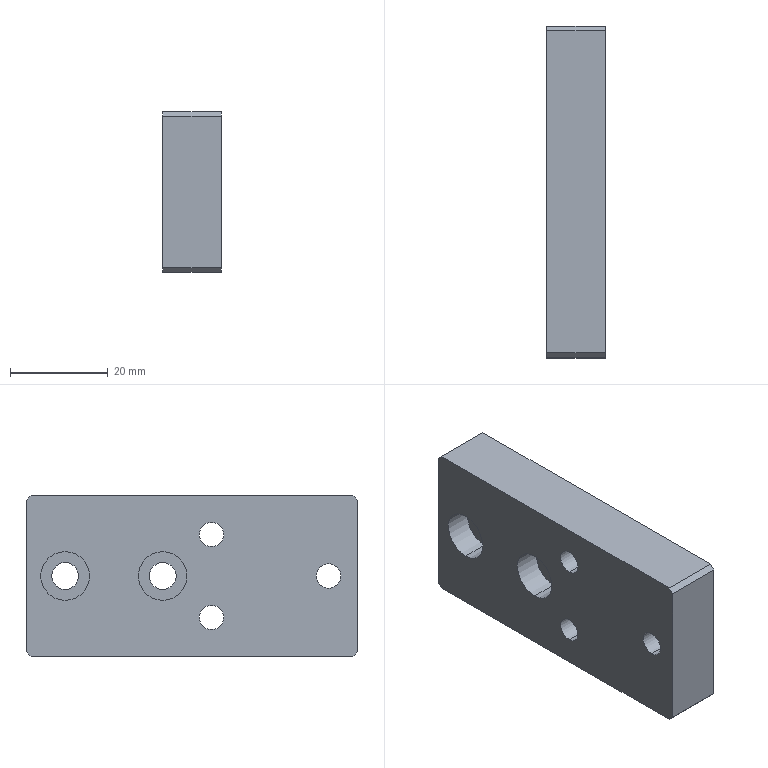Part | SolidWorks | features HoleWzd 3, Chamfer 1, Extrusion 1 | 1 solid | 34 faces | box 12 x 68 x 33 mm | volume 24708 mm3 | cylinder 18 | plane 12 | cone 4 | commonest cylinder face diameters 5 x6 4.2 x4 5.5 x4 10 x4
STEP:
#1=CARTESIAN_POINT('',(-70.982,-19.604,-21.5));
#2=VERTEX_POINT('',#1);
#3=CARTESIAN_POINT('',(-70.982,-19.604,-11.5));
#4=VERTEX_POINT('',#3);
#5=CARTESIAN_POINT('',(-70.982,-19.604,-16.5));
#6=DIRECTION('',(-1.,0.,0.));
#7=DIRECTION('',(0.,0.,1.));
#8=AXIS2_PLACEMENT_3D('',#5,#6,#7);
#9=CIRCLE('',#8,5.);
#10=EDGE_CURVE('',#2,#4,#9,.T.);
#11=ORIENTED_EDGE('',*,*,#10,.F.);
#12=CARTESIAN_POINT('',(-76.482,-19.604,-21.5));
#13=VERTEX_POINT('',#12);
#14=CARTESIAN_POINT('',(-76.482,-19.604,-21.5));
#15=DIRECTION('',(-1.,0.,0.));
#16=VECTOR('',#15,1000.);
#17=LINE('',#14,#16);
#18=EDGE_CURVE('',#2,#13,#17,.T.);
#19=ORIENTED_EDGE('',*,*,#18,.T.);
#20=CARTESIAN_POINT('',(-76.482,-19.604,-11.5));
#21=VERTEX_POINT('',#20);
#22=CARTESIAN_POINT('',(-76.482,-19.604,-16.5));
#23=DIRECTION('',(-1.,0.,0.));
#24=DIRECTION('',(0.,0.,1.));
#25=AXIS2_PLACEMENT_3D('',#22,#23,#24);
#26=CIRCLE('',#25,5.);
#27=EDGE_CURVE('',#13,#21,#26,.T.);
#28=ORIENTED_EDGE('',*,*,#27,.T.);
#29=CARTESIAN_POINT('',(-76.482,-19.604,-11.5));
#30=DIRECTION('',(-1.,0.,0.));
#31=VECTOR('',#30,1000.);
#32=LINE('',#29,#31);
#33=EDGE_CURVE('',#4,#21,#32,.T.);
#34=ORIENTED_EDGE('',*,*,#33,.F.);
#35=EDGE_LOOP('',(#11,#19,#28,#34));
#36=FACE_OUTER_BOUND('',#35,.T.);
#37=CARTESIAN_POINT('',(-76.482,-19.604,-16.5));
#38=DIRECTION('',(-1.,0.,0.));
#39=DIRECTION('',(0.,0.,1.));
#40=AXIS2_PLACEMENT_3D('',#37,#38,#39);
#41=CYLINDRICAL_SURFACE('',#40,5.);
#42=ADVANCED_FACE('',(#36),#41,.F.);
#43=CARTESIAN_POINT('',(-64.482,-19.604,-19.25));
#44=VERTEX_POINT('',#43);
#45=CARTESIAN_POINT('',(-64.482,-19.604,-13.75));
#46=VERTEX_POINT('',#45);
#47=CARTESIAN_POINT('',(-64.482,-19.604,-16.5));
#48=DIRECTION('',(-1.,0.,0.));
#49=DIRECTION('',(0.,0.,1.));
#50=AXIS2_PLACEMENT_3D('',#47,#48,#49);
#51=CIRCLE('',#50,2.75);
#52=EDGE_CURVE('',#44,#46,#51,.T.);
#53=ORIENTED_EDGE('',*,*,#52,.F.);
#54=CARTESIAN_POINT('',(-70.982,-19.604,-19.25));
#55=VERTEX_POINT('',#54);
#56=CARTESIAN_POINT('',(-76.482,-19.604,-19.25));
#57=DIRECTION('',(-1.,0.,0.));
#58=VECTOR('',#57,1000.);
#59=LINE('',#56,#58);
#60=EDGE_CURVE('',#44,#55,#59,.T.);
#61=ORIENTED_EDGE('',*,*,#60,.T.);
#62=CARTESIAN_POINT('',(-70.982,-19.604,-13.75));
#63=VERTEX_POINT('',#62);
#64=CARTESIAN_POINT('',(-70.982,-19.604,-16.5));
#65=DIRECTION('',(-1.,0.,0.));
#66=DIRECTION('',(0.,0.,1.));
#67=AXIS2_PLACEMENT_3D('',#64,#65,#66);
#68=CIRCLE('',#67,2.75);
#69=EDGE_CURVE('',#55,#63,#68,.T.);
#70=ORIENTED_EDGE('',*,*,#69,.T.);
#71=CARTESIAN_POINT('',(-76.482,-19.604,-13.75));
#72=DIRECTION('',(-1.,0.,0.));
#73=VECTOR('',#72,1000.);
#74=LINE('',#71,#73);
#75=EDGE_CURVE('',#46,#63,#74,.T.);
#76=ORIENTED_EDGE('',*,*,#75,.F.);
#77=EDGE_LOOP('',(#53,#61,#70,#76));
#78=FACE_OUTER_BOUND('',#77,.T.);
#79=CARTESIAN_POINT('',(-76.482,-19.604,-16.5));
#80=DIRECTION('',(-1.,0.,0.));
#81=DIRECTION('',(0.,0.,1.));
#82=AXIS2_PLACEMENT_3D('',#79,#80,#81);
#83=CYLINDRICAL_SURFACE('',#82,2.75);
#84=ADVANCED_FACE('',(#78),#83,.F.);
#85=CARTESIAN_POINT('',(-70.982,-39.608,-21.5));
#86=VERTEX_POINT('',#85);
#87=CARTESIAN_POINT('',(-70.982,-39.608,-11.5));
#88=VERTEX_POINT('',#87);
#89=CARTESIAN_POINT('',(-70.982,-39.608,-16.5));
#90=DIRECTION('',(-1.,0.,0.));
#91=DIRECTION('',(0.,0.,1.));
#92=AXIS2_PLACEMENT_3D('',#89,#90,#91);
#93=CIRCLE('',#92,5.);
#94=EDGE_CURVE('',#86,#88,#93,.T.);
#95=ORIENTED_EDGE('',*,*,#94,.F.);
#96=CARTESIAN_POINT('',(-76.482,-39.608,-21.5));
#97=VERTEX_POINT('',#96);
#98=CARTESIAN_POINT('',(-76.482,-39.608,-21.5));
#99=DIRECTION('',(-1.,0.,0.));
#100=VECTOR('',#99,1000.);
#101=LINE('',#98,#100);
#102=EDGE_CURVE('',#86,#97,#101,.T.);
#103=ORIENTED_EDGE('',*,*,#102,.T.);
#104=CARTESIAN_POINT('',(-76.482,-39.608,-11.5));
#105=VERTEX_POINT('',#104);
#106=CARTESIAN_POINT('',(-76.482,-39.608,-16.5));
#107=DIRECTION('',(-1.,0.,0.));
#108=DIRECTION('',(0.,0.,1.));
#109=AXIS2_PLACEMENT_3D('',#106,#107,#108);
#110=CIRCLE('',#109,5.);
#111=EDGE_CURVE('',#97,#105,#110,.T.);
#112=ORIENTED_EDGE('',*,*,#111,.T.);
#113=CARTESIAN_POINT('',(-76.482,-39.608,-11.5));
#114=DIRECTION('',(-1.,0.,0.));
#115=VECTOR('',#114,1000.);
#116=LINE('',#113,#115);
#117=EDGE_CURVE('',#88,#105,#116,.T.);
#118=ORIENTED_EDGE('',*,*,#117,.F.);
#119=EDGE_LOOP('',(#95,#103,#112,#118));
#120=FACE_OUTER_BOUND('',#119,.T.);
#121=CARTESIAN_POINT('',(-76.482,-39.608,-16.5));
#122=DIRECTION('',(-1.,0.,0.));
#123=DIRECTION('',(0.,0.,1.));
#124=AXIS2_PLACEMENT_3D('',#121,#122,#123);
#125=CYLINDRICAL_SURFACE('',#124,5.);
#126=ADVANCED_FACE('',(#120),#125,.F.);
#127=CARTESIAN_POINT('',(-64.482,-39.608,-19.25));
#128=VERTEX_POINT('',#127);
#129=CARTESIAN_POINT('',(-64.482,-39.608,-13.75));
#130=VERTEX_POINT('',#129);
#131=CARTESIAN_POINT('',(-64.482,-39.608,-16.5));
#132=DIRECTION('',(-1.,0.,0.));
#133=DIRECTION('',(0.,0.,1.));
#134=AXIS2_PLACEMENT_3D('',#131,#132,#133);
#135=CIRCLE('',#134,2.75);
#136=EDGE_CURVE('',#128,#130,#135,.T.);
#137=ORIENTED_EDGE('',*,*,#136,.F.);
#138=CARTESIAN_POINT('',(-70.982,-39.608,-19.25));
#139=VERTEX_POINT('',#138);
#140=CARTESIAN_POINT('',(-76.482,-39.608,-19.25));
#141=DIRECTION('',(-1.,0.,0.));
#142=VECTOR('',#141,1000.);
#143=LINE('',#140,#142);
#144=EDGE_CURVE('',#128,#139,#143,.T.);
#145=ORIENTED_EDGE('',*,*,#144,.T.);
#146=CARTESIAN_POINT('',(-70.982,-39.608,-13.75));
#147=VERTEX_POINT('',#146);
#148=CARTESIAN_POINT('',(-70.982,-39.608,-16.5));
#149=DIRECTION('',(-1.,0.,0.));
#150=DIRECTION('',(0.,0.,1.));
#151=AXIS2_PLACEMENT_3D('',#148,#149,#150);
#152=CIRCLE('',#151,2.75);
#153=EDGE_CURVE('',#139,#147,#152,.T.);
#154=ORIENTED_EDGE('',*,*,#153,.T.);
#155=CARTESIAN_POINT('',(-76.482,-39.608,-13.75));
#156=DIRECTION('',(-1.,0.,0.));
#157=VECTOR('',#156,1000.);
#158=LINE('',#155,#157);
#159=EDGE_CURVE('',#130,#147,#158,.T.);
#160=ORIENTED_EDGE('',*,*,#159,.F.);
#161=EDGE_LOOP('',(#137,#145,#154,#160));
#162=FACE_OUTER_BOUND('',#161,.T.);
#163=CARTESIAN_POINT('',(-76.482,-39.608,-16.5));
#164=DIRECTION('',(-1.,0.,0.));
#165=DIRECTION('',(0.,0.,1.));
#166=AXIS2_PLACEMENT_3D('',#163,#164,#165);
#167=CYLINDRICAL_SURFACE('',#166,2.75);
#168=ADVANCED_FACE('',(#162),#167,.F.);
#169=CARTESIAN_POINT('',(-70.482,-22.608,-28.1));
#170=VERTEX_POINT('',#169);
#171=CARTESIAN_POINT('',(-70.482,-22.608,-23.9));
#172=VERTEX_POINT('',#171);
#173=CARTESIAN_POINT('',(-70.482,-22.608,-26.));
#174=DIRECTION('',(0.,1.,0.));
#175=DIRECTION('',(0.,0.,1.));
#176=AXIS2_PLACEMENT_3D('',#173,#174,#175);
#177=CIRCLE('',#176,2.1);
#178=EDGE_CURVE('',#170,#172,#177,.T.);
#179=ORIENTED_EDGE('',*,*,#178,.F.);
#180=CARTESIAN_POINT('',(-70.482,-11.608,-28.1));
#181=VERTEX_POINT('',#180);
#182=CARTESIAN_POINT('',(-70.482,-11.608,-28.1));
#183=DIRECTION('',(0.,1.,0.));
#184=VECTOR('',#183,1000.);
#185=LINE('',#182,#184);
#186=EDGE_CURVE('',#170,#181,#185,.T.);
#187=ORIENTED_EDGE('',*,*,#186,.T.);
#188=CARTESIAN_POINT('',(-70.482,-11.608,-23.9));
#189=VERTEX_POINT('',#188);
#190=CARTESIAN_POINT('',(-70.482,-11.608,-26.));
#191=DIRECTION('',(0.,1.,0.));
#192=DIRECTION('',(0.,0.,1.));
#193=AXIS2_PLACEMENT_3D('',#190,#191,#192);
#194=CIRCLE('',#193,2.1);
#195=EDGE_CURVE('',#181,#189,#194,.T.);
#196=ORIENTED_EDGE('',*,*,#195,.T.);
#197=CARTESIAN_POINT('',(-70.482,-11.608,-23.9));
#198=DIRECTION('',(0.,1.,0.));
#199=VECTOR('',#198,1000.);
#200=LINE('',#197,#199);
#201=EDGE_CURVE('',#172,#189,#200,.T.);
#202=ORIENTED_EDGE('',*,*,#201,.F.);
#203=EDGE_LOOP('',(#179,#187,#196,#202));
#204=FACE_OUTER_BOUND('',#203,.T.);
#205=CARTESIAN_POINT('',(-70.482,-11.608,-26.));
#206=DIRECTION('',(0.,1.,0.));
#207=DIRECTION('',(0.,0.,1.));
#208=AXIS2_PLACEMENT_3D('',#205,#206,#207);
#209=CYLINDRICAL_SURFACE('',#208,2.1);
#210=ADVANCED_FACE('',(#204),#209,.F.);
#211=CARTESIAN_POINT('',(-70.482,-23.87,-26.));
#212=VERTEX_POINT('',#211);
#213=CARTESIAN_POINT('',(-70.482,-22.608,-23.9));
#214=DIRECTION('',(0.,0.515,0.8572));
#215=VECTOR('',#214,1000.);
#216=LINE('',#213,#215);
#217=EDGE_CURVE('',#212,#172,#216,.T.);
#218=ORIENTED_EDGE('',*,*,#217,.F.);
#219=CARTESIAN_POINT('',(-70.482,-22.608,-28.1));
#220=DIRECTION('',(0.,0.515,-0.8572));
#221=VECTOR('',#220,1000.);
#222=LINE('',#219,#221);
#223=EDGE_CURVE('',#212,#170,#222,.T.);
#224=ORIENTED_EDGE('',*,*,#223,.T.);
#225=ORIENTED_EDGE('',*,*,#178,.T.);
#226=EDGE_LOOP('',(#218,#224,#225));
#227=FACE_OUTER_BOUND('',#226,.T.);
#228=CARTESIAN_POINT('',(-70.482,-22.608,-26.));
#229=DIRECTION('',(0.,1.,0.));
#230=DIRECTION('',(0.,0.,1.));
#231=AXIS2_PLACEMENT_3D('',#228,#229,#230);
#232=CONICAL_SURFACE('',#231,2.1,1.03);
#233=ADVANCED_FACE('',(#227),#232,.F.);
#234=CARTESIAN_POINT('',(-70.482,-22.608,-9.1));
#235=VERTEX_POINT('',#234);
#236=CARTESIAN_POINT('',(-70.482,-22.608,-4.9));
#237=VERTEX_POINT('',#236);
#238=CARTESIAN_POINT('',(-70.482,-22.608,-7.));
#239=DIRECTION('',(0.,1.,0.));
#240=DIRECTION('',(0.,0.,1.));
#241=AXIS2_PLACEMENT_3D('',#238,#239,#240);
#242=CIRCLE('',#241,2.1);
#243=EDGE_CURVE('',#235,#237,#242,.T.);
#244=ORIENTED_EDGE('',*,*,#243,.F.);
#245=CARTESIAN_POINT('',(-70.482,-11.608,-9.1));
#246=VERTEX_POINT('',#245);
#247=CARTESIAN_POINT('',(-70.482,-11.608,-9.1));
#248=DIRECTION('',(0.,1.,0.));
#249=VECTOR('',#248,1000.);
#250=LINE('',#247,#249);
#251=EDGE_CURVE('',#235,#246,#250,.T.);
#252=ORIENTED_EDGE('',*,*,#251,.T.);
#253=CARTESIAN_POINT('',(-70.482,-11.608,-4.9));
#254=VERTEX_POINT('',#253);
#255=CARTESIAN_POINT('',(-70.482,-11.608,-7.));
#256=DIRECTION('',(0.,1.,0.));
#257=DIRECTION('',(0.,0.,1.));
#258=AXIS2_PLACEMENT_3D('',#255,#256,#257);
#259=CIRCLE('',#258,2.1);
#260=EDGE_CURVE('',#246,#254,#259,.T.);
#261=ORIENTED_EDGE('',*,*,#260,.T.);
#262=CARTESIAN_POINT('',(-70.482,-11.608,-4.9));
#263=DIRECTION('',(0.,1.,0.));
#264=VECTOR('',#263,1000.);
#265=LINE('',#262,#264);
#266=EDGE_CURVE('',#237,#254,#265,.T.);
#267=ORIENTED_EDGE('',*,*,#266,.F.);
#268=EDGE_LOOP('',(#244,#252,#261,#267));
#269=FACE_OUTER_BOUND('',#268,.T.);
#270=CARTESIAN_POINT('',(-70.482,-11.608,-7.));
#271=DIRECTION('',(0.,1.,0.));
#272=DIRECTION('',(0.,0.,1.));
#273=AXIS2_PLACEMENT_3D('',#270,#271,#272);
#274=CYLINDRICAL_SURFACE('',#273,2.1);
#275=ADVANCED_FACE('',(#269),#274,.F.);
#276=CARTESIAN_POINT('',(-70.482,-23.87,-7.));
#277=VERTEX_POINT('',#276);
#278=CARTESIAN_POINT('',(-70.482,-22.608,-4.9));
#279=DIRECTION('',(0.,0.515,0.8572));
#280=VECTOR('',#279,1000.);
#281=LINE('',#278,#280);
#282=EDGE_CURVE('',#277,#237,#281,.T.);
#283=ORIENTED_EDGE('',*,*,#282,.F.);
#284=CARTESIAN_POINT('',(-70.482,-22.608,-9.1));
#285=DIRECTION('',(0.,0.515,-0.8572));
#286=VECTOR('',#285,1000.);
#287=LINE('',#284,#286);
#288=EDGE_CURVE('',#277,#235,#287,.T.);
#289=ORIENTED_EDGE('',*,*,#288,.T.);
#290=ORIENTED_EDGE('',*,*,#243,.T.);
#291=EDGE_LOOP('',(#283,#289,#290));
#292=FACE_OUTER_BOUND('',#291,.T.);
#293=CARTESIAN_POINT('',(-70.482,-22.608,-7.));
#294=DIRECTION('',(0.,1.,0.));
#295=DIRECTION('',(0.,0.,1.));
#296=AXIS2_PLACEMENT_3D('',#293,#294,#295);
#297=CONICAL_SURFACE('',#296,2.1,1.03);
#298=ADVANCED_FACE('',(#292),#297,.F.);
#299=CARTESIAN_POINT('',(-64.482,-73.608,-14.));
#300=VERTEX_POINT('',#299);
#301=CARTESIAN_POINT('',(-64.482,-73.608,-19.));
#302=VERTEX_POINT('',#301);
#303=CARTESIAN_POINT('',(-64.482,-73.608,-16.5));
#304=DIRECTION('',(1.,0.,0.));
#305=DIRECTION('',(0.,0.,-1.));
#306=AXIS2_PLACEMENT_3D('',#303,#304,#305);
#307=CIRCLE('',#306,2.5);
#308=EDGE_CURVE('',#300,#302,#307,.T.);
#309=ORIENTED_EDGE('',*,*,#308,.T.);
#310=CARTESIAN_POINT('',(-76.482,-73.608,-19.));
#311=VERTEX_POINT('',#310);
#312=CARTESIAN_POINT('',(-76.482,-73.608,-19.));
#313=DIRECTION('',(-1.,0.,0.));
#314=VECTOR('',#313,1000.);
#315=LINE('',#312,#314);
#316=EDGE_CURVE('',#302,#311,#315,.T.);
#317=ORIENTED_EDGE('',*,*,#316,.T.);
#318=CARTESIAN_POINT('',(-76.482,-73.608,-14.));
#319=VERTEX_POINT('',#318);
#320=CARTESIAN_POINT('',(-76.482,-73.608,-16.5));
#321=DIRECTION('',(-1.,0.,0.));
#322=DIRECTION('',(0.,0.,1.));
#323=AXIS2_PLACEMENT_3D('',#320,#321,#322);
#324=CIRCLE('',#323,2.5);
#325=EDGE_CURVE('',#311,#319,#324,.T.);
#326=ORIENTED_EDGE('',*,*,#325,.T.);
#327=CARTESIAN_POINT('',(-76.482,-73.608,-14.));
#328=DIRECTION('',(-1.,0.,0.));
#329=VECTOR('',#328,1000.);
#330=LINE('',#327,#329);
#331=EDGE_CURVE('',#300,#319,#330,.T.);
#332=ORIENTED_EDGE('',*,*,#331,.F.);
#333=EDGE_LOOP('',(#309,#317,#326,#332));
#334=FACE_OUTER_BOUND('',#333,.T.);
#335=CARTESIAN_POINT('',(-76.482,-73.608,-16.5));
#336=DIRECTION('',(-1.,0.,0.));
#337=DIRECTION('',(0.,0.,1.));
#338=AXIS2_PLACEMENT_3D('',#335,#336,#337);
#339=CYLINDRICAL_SURFACE('',#338,2.5);
#340=ADVANCED_FACE('',(#334),#339,.F.);
#341=CARTESIAN_POINT('',(-64.482,-49.608,-5.5));
#342=VERTEX_POINT('',#341);
#343=CARTESIAN_POINT('',(-64.482,-49.608,-10.5));
#344=VERTEX_POINT('',#343);
#345=CARTESIAN_POINT('',(-64.482,-49.608,-8.));
#346=DIRECTION('',(1.,0.,0.));
#347=DIRECTION('',(0.,0.,-1.));
#348=AXIS2_PLACEMENT_3D('',#345,#346,#347);
#349=CIRCLE('',#348,2.5);
#350=EDGE_CURVE('',#342,#344,#349,.T.);
#351=ORIENTED_EDGE('',*,*,#350,.T.);
#352=CARTESIAN_POINT('',(-76.482,-49.608,-10.5));
#353=VERTEX_POINT('',#352);
#354=CARTESIAN_POINT('',(-76.482,-49.608,-10.5));
#355=DIRECTION('',(-1.,0.,0.));
#356=VECTOR('',#355,1000.);
#357=LINE('',#354,#356);
#358=EDGE_CURVE('',#344,#353,#357,.T.);
#359=ORIENTED_EDGE('',*,*,#358,.T.);
#360=CARTESIAN_POINT('',(-76.482,-49.608,-5.5));
#361=VERTEX_POINT('',#360);
#362=CARTESIAN_POINT('',(-76.482,-49.608,-8.));
#363=DIRECTION('',(-1.,0.,0.));
#364=DIRECTION('',(0.,0.,1.));
#365=AXIS2_PLACEMENT_3D('',#362,#363,#364);
#366=CIRCLE('',#365,2.5);
#367=EDGE_CURVE('',#353,#361,#366,.T.);
#368=ORIENTED_EDGE('',*,*,#367,.T.);
#369=CARTESIAN_POINT('',(-76.482,-49.608,-5.5));
#370=DIRECTION('',(-1.,0.,0.));
#371=VECTOR('',#370,1000.);
#372=LINE('',#369,#371);
#373=EDGE_CURVE('',#342,#361,#372,.T.);
#374=ORIENTED_EDGE('',*,*,#373,.F.);
#375=EDGE_LOOP('',(#351,#359,#368,#374));
#376=FACE_OUTER_BOUND('',#375,.T.);
#377=CARTESIAN_POINT('',(-76.482,-49.608,-8.));
#378=DIRECTION('',(-1.,0.,0.));
#379=DIRECTION('',(0.,0.,1.));
#380=AXIS2_PLACEMENT_3D('',#377,#378,#379);
#381=CYLINDRICAL_SURFACE('',#380,2.5);
#382=ADVANCED_FACE('',(#376),#381,.F.);
#383=CARTESIAN_POINT('',(-64.482,-49.608,-22.5));
#384=VERTEX_POINT('',#383);
#385=CARTESIAN_POINT('',(-64.482,-49.608,-27.5));
#386=VERTEX_POINT('',#385);
#387=CARTESIAN_POINT('',(-64.482,-49.608,-25.));
#388=DIRECTION('',(1.,0.,0.));
#389=DIRECTION('',(0.,0.,-1.));
#390=AXIS2_PLACEMENT_3D('',#387,#388,#389);
#391=CIRCLE('',#390,2.5);
#392=EDGE_CURVE('',#384,#386,#391,.T.);
#393=ORIENTED_EDGE('',*,*,#392,.T.);
#394=CARTESIAN_POINT('',(-76.482,-49.608,-27.5));
#395=VERTEX_POINT('',#394);
#396=CARTESIAN_POINT('',(-76.482,-49.608,-27.5));
#397=DIRECTION('',(-1.,0.,0.));
#398=VECTOR('',#397,1000.);
#399=LINE('',#396,#398);
#400=EDGE_CURVE('',#386,#395,#399,.T.);
#401=ORIENTED_EDGE('',*,*,#400,.T.);
#402=CARTESIAN_POINT('',(-76.482,-49.608,-22.5));
#403=VERTEX_POINT('',#402);
#404=CARTESIAN_POINT('',(-76.482,-49.608,-25.));
#405=DIRECTION('',(-1.,0.,0.));
#406=DIRECTION('',(0.,0.,1.));
#407=AXIS2_PLACEMENT_3D('',#404,#405,#406);
#408=CIRCLE('',#407,2.5);
#409=EDGE_CURVE('',#395,#403,#408,.T.);
#410=ORIENTED_EDGE('',*,*,#409,.T.);
#411=CARTESIAN_POINT('',(-76.482,-49.608,-22.5));
#412=DIRECTION('',(-1.,0.,0.));
#413=VECTOR('',#412,1000.);
#414=LINE('',#411,#413);
#415=EDGE_CURVE('',#384,#403,#414,.T.);
#416=ORIENTED_EDGE('',*,*,#415,.F.);
#417=EDGE_LOOP('',(#393,#401,#410,#416));
#418=FACE_OUTER_BOUND('',#417,.T.);
#419=CARTESIAN_POINT('',(-76.482,-49.608,-25.));
#420=DIRECTION('',(-1.,0.,0.));
#421=DIRECTION('',(0.,0.,1.));
#422=AXIS2_PLACEMENT_3D('',#419,#420,#421);
#423=CYLINDRICAL_SURFACE('',#422,2.5);
#424=ADVANCED_FACE('',(#418),#423,.F.);
#425=CARTESIAN_POINT('',(-76.482,-19.604,-16.5));
#426=DIRECTION('',(-1.,0.,0.));
#427=DIRECTION('',(0.,0.,1.));
#428=AXIS2_PLACEMENT_3D('',#425,#426,#427);
#429=CIRCLE('',#428,5.);
#430=EDGE_CURVE('',#21,#13,#429,.T.);
#431=ORIENTED_EDGE('',*,*,#430,.F.);
#432=ORIENTED_EDGE('',*,*,#27,.F.);
#433=EDGE_LOOP('',(#431,#432));
#434=FACE_BOUND('',#433,.T.);
#435=CARTESIAN_POINT('',(-76.482,-39.608,-16.5));
#436=DIRECTION('',(-1.,0.,0.));
#437=DIRECTION('',(0.,0.,1.));
#438=AXIS2_PLACEMENT_3D('',#435,#436,#437);
#439=CIRCLE('',#438,5.);
#440=EDGE_CURVE('',#105,#97,#439,.T.);
#441=ORIENTED_EDGE('',*,*,#440,.F.);
#442=ORIENTED_EDGE('',*,*,#111,.F.);
#443=EDGE_LOOP('',(#441,#442));
#444=FACE_BOUND('',#443,.T.);
#445=CARTESIAN_POINT('',(-76.482,-73.608,-16.5));
#446=DIRECTION('',(-1.,0.,0.));
#447=DIRECTION('',(0.,0.,1.));
#448=AXIS2_PLACEMENT_3D('',#445,#446,#447);
#449=CIRCLE('',#448,2.5);
#450=EDGE_CURVE('',#319,#311,#449,.T.);
#451=ORIENTED_EDGE('',*,*,#450,.F.);
#452=ORIENTED_EDGE('',*,*,#325,.F.);
#453=EDGE_LOOP('',(#451,#452));
#454=FACE_BOUND('',#453,.T.);
#455=CARTESIAN_POINT('',(-76.482,-49.608,-8.));
#456=DIRECTION('',(-1.,0.,0.));
#457=DIRECTION('',(0.,0.,1.));
#458=AXIS2_PLACEMENT_3D('',#455,#456,#457);
#459=CIRCLE('',#458,2.5);
#460=EDGE_CURVE('',#361,#353,#459,.T.);
#461=ORIENTED_EDGE('',*,*,#460,.F.);
#462=ORIENTED_EDGE('',*,*,#367,.F.);
#463=EDGE_LOOP('',(#461,#462));
#464=FACE_BOUND('',#463,.T.);
#465=CARTESIAN_POINT('',(-76.482,-49.608,-25.));
#466=DIRECTION('',(-1.,0.,0.));
#467=DIRECTION('',(0.,0.,1.));
#468=AXIS2_PLACEMENT_3D('',#465,#466,#467);
#469=CIRCLE('',#468,2.5);
#470=EDGE_CURVE('',#403,#395,#469,.T.);
#471=ORIENTED_EDGE('',*,*,#470,.F.);
#472=ORIENTED_EDGE('',*,*,#409,.F.);
#473=EDGE_LOOP('',(#471,#472));
#474=FACE_BOUND('',#473,.T.);
#475=CARTESIAN_POINT('',(-76.482,-12.608,0.));
#476=VERTEX_POINT('',#475);
#477=CARTESIAN_POINT('',(-76.482,-78.608,0.));
#478=VERTEX_POINT('',#477);
#479=CARTESIAN_POINT('',(-76.482,-79.608,0.));
#480=DIRECTION('',(0.,-1.,0.));
#481=VECTOR('',#480,1000.);
#482=LINE('',#479,#481);
#483=EDGE_CURVE('',#476,#478,#482,.T.);
#484=ORIENTED_EDGE('',*,*,#483,.F.);
#485=CARTESIAN_POINT('',(-76.482,-11.608,-1.));
#486=VERTEX_POINT('',#485);
#487=CARTESIAN_POINT('',(-76.482,-29.608,17.));
#488=DIRECTION('',(0.,0.7071,-0.7071));
#489=VECTOR('',#488,1000.);
#490=LINE('',#487,#489);
#491=EDGE_CURVE('',#476,#486,#490,.T.);
#492=ORIENTED_EDGE('',*,*,#491,.T.);
#493=CARTESIAN_POINT('',(-76.482,-11.608,-32.));
#494=VERTEX_POINT('',#493);
#495=CARTESIAN_POINT('',(-76.482,-11.608,-33.));
#496=DIRECTION('',(0.,0.,1.));
#497=VECTOR('',#496,1000.);
#498=LINE('',#495,#497);
#499=EDGE_CURVE('',#494,#486,#498,.T.);
#500=ORIENTED_EDGE('',*,*,#499,.F.);
#501=CARTESIAN_POINT('',(-76.482,-12.608,-33.));
#502=VERTEX_POINT('',#501);
#503=CARTESIAN_POINT('',(-76.482,-46.108,-66.5));
#504=DIRECTION('',(0.,-0.7071,-0.7071));
#505=VECTOR('',#504,1000.);
#506=LINE('',#503,#505);
#507=EDGE_CURVE('',#494,#502,#506,.T.);
#508=ORIENTED_EDGE('',*,*,#507,.T.);
#509=CARTESIAN_POINT('',(-76.482,-78.608,-33.));
#510=VERTEX_POINT('',#509);
#511=CARTESIAN_POINT('',(-76.482,-79.608,-33.));
#512=DIRECTION('',(0.,-1.,0.));
#513=VECTOR('',#512,1000.);
#514=LINE('',#511,#513);
#515=EDGE_CURVE('',#502,#510,#514,.T.);
#516=ORIENTED_EDGE('',*,*,#515,.T.);
#517=CARTESIAN_POINT('',(-76.482,-79.608,-32.));
#518=VERTEX_POINT('',#517);
#519=CARTESIAN_POINT('',(-76.482,-79.108,-32.5));
#520=DIRECTION('',(0.,-0.7071,0.7071));
#521=VECTOR('',#520,1000.);
#522=LINE('',#519,#521);
#523=EDGE_CURVE('',#510,#518,#522,.T.);
#524=ORIENTED_EDGE('',*,*,#523,.T.);
#525=CARTESIAN_POINT('',(-76.482,-79.608,-1.));
#526=VERTEX_POINT('',#525);
#527=CARTESIAN_POINT('',(-76.482,-79.608,-33.));
#528=DIRECTION('',(0.,0.,1.));
#529=VECTOR('',#528,1000.);
#530=LINE('',#527,#529);
#531=EDGE_CURVE('',#518,#526,#530,.T.);
#532=ORIENTED_EDGE('',*,*,#531,.T.);
#533=CARTESIAN_POINT('',(-76.482,-95.608,-17.));
#534=DIRECTION('',(0.,0.7071,0.7071));
#535=VECTOR('',#534,1000.);
#536=LINE('',#533,#535);
#537=EDGE_CURVE('',#526,#478,#536,.T.);
#538=ORIENTED_EDGE('',*,*,#537,.T.);
#539=EDGE_LOOP('',(#484,#492,#500,#508,#516,#524,#532,#538));
#540=FACE_OUTER_BOUND('',#539,.T.);
#541=CARTESIAN_POINT('',(-76.482,-79.608,-33.));
#542=DIRECTION('',(-1.,0.,0.));
#543=DIRECTION('',(0.,0.,1.));
#544=AXIS2_PLACEMENT_3D('',#541,#542,#543);
#545=PLANE('',#544);
#546=ADVANCED_FACE('',(#434,#444,#454,#464,#474,#540),#545,.T.);
#547=CARTESIAN_POINT('',(-70.482,-11.608,-26.));
#548=DIRECTION('',(0.,1.,0.));
#549=DIRECTION('',(0.,0.,1.));
#550=AXIS2_PLACEMENT_3D('',#547,#548,#549);
#551=CIRCLE('',#550,2.1);
#552=EDGE_CURVE('',#189,#181,#551,.T.);
#553=ORIENTED_EDGE('',*,*,#552,.F.);
#554=ORIENTED_EDGE('',*,*,#195,.F.);
#555=EDGE_LOOP('',(#553,#554));
#556=FACE_BOUND('',#555,.T.);
#557=CARTESIAN_POINT('',(-70.482,-11.608,-7.));
#558=DIRECTION('',(0.,1.,0.));
#559=DIRECTION('',(0.,0.,1.));
#560=AXIS2_PLACEMENT_3D('',#557,#558,#559);
#561=CIRCLE('',#560,2.1);
#562=EDGE_CURVE('',#254,#246,#561,.T.);
#563=ORIENTED_EDGE('',*,*,#562,.F.);
#564=ORIENTED_EDGE('',*,*,#260,.F.);
#565=EDGE_LOOP('',(#563,#564));
#566=FACE_BOUND('',#565,.T.);
#567=ORIENTED_EDGE('',*,*,#499,.T.);
#568=CARTESIAN_POINT('',(-64.482,-11.608,-1.));
#569=VERTEX_POINT('',#568);
#570=CARTESIAN_POINT('',(-64.482,-11.608,-1.));
#571=DIRECTION('',(1.,0.,0.));
#572=VECTOR('',#571,1000.);
#573=LINE('',#570,#572);
#574=EDGE_CURVE('',#486,#569,#573,.T.);
#575=ORIENTED_EDGE('',*,*,#574,.T.);
#576=CARTESIAN_POINT('',(-64.482,-11.608,-32.));
#577=VERTEX_POINT('',#576);
#578=CARTESIAN_POINT('',(-64.482,-11.608,-33.));
#579=DIRECTION('',(0.,0.,1.));
#580=VECTOR('',#579,1000.);
#581=LINE('',#578,#580);
#582=EDGE_CURVE('',#577,#569,#581,.T.);
#583=ORIENTED_EDGE('',*,*,#582,.F.);
#584=CARTESIAN_POINT('',(-76.482,-11.608,-32.));
#585=DIRECTION('',(-1.,0.,0.));
#586=VECTOR('',#585,1000.);
#587=LINE('',#584,#586);
#588=EDGE_CURVE('',#577,#494,#587,.T.);
#589=ORIENTED_EDGE('',*,*,#588,.T.);
#590=EDGE_LOOP('',(#567,#575,#583,#589));
#591=FACE_OUTER_BOUND('',#590,.T.);
#592=CARTESIAN_POINT('',(-76.482,-11.608,-33.));
#593=DIRECTION('',(0.,1.,0.));
#594=DIRECTION('',(-1.,0.,0.));
#595=AXIS2_PLACEMENT_3D('',#592,#593,#594);
#596=PLANE('',#595);
#597=ADVANCED_FACE('',(#556,#566,#591),#596,.T.);
#598=CARTESIAN_POINT('',(-64.482,-19.604,-16.5));
#599=DIRECTION('',(-1.,0.,0.));
#600=DIRECTION('',(0.,0.,1.));
#601=AXIS2_PLACEMENT_3D('',#598,#599,#600);
#602=CIRCLE('',#601,2.75);
#603=EDGE_CURVE('',#46,#44,#602,.T.);
#604=ORIENTED_EDGE('',*,*,#603,.T.);
#605=ORIENTED_EDGE('',*,*,#52,.T.);
#606=EDGE_LOOP('',(#604,#605));
#607=FACE_BOUND('',#606,.T.);
#608=CARTESIAN_POINT('',(-64.482,-39.608,-16.5));
#609=DIRECTION('',(-1.,0.,0.));
#610=DIRECTION('',(0.,0.,1.));
#611=AXIS2_PLACEMENT_3D('',#608,#609,#610);
#612=CIRCLE('',#611,2.75);
#613=EDGE_CURVE('',#130,#128,#612,.T.);
#614=ORIENTED_EDGE('',*,*,#613,.T.);
#615=ORIENTED_EDGE('',*,*,#136,.T.);
#616=EDGE_LOOP('',(#614,#615));
#617=FACE_BOUND('',#616,.T.);
#618=ORIENTED_EDGE('',*,*,#308,.F.);
#619=CARTESIAN_POINT('',(-64.482,-73.608,-16.5));
#620=DIRECTION('',(1.,0.,0.));
#621=DIRECTION('',(0.,0.,-1.));
#622=AXIS2_PLACEMENT_3D('',#619,#620,#621);
#623=CIRCLE('',#622,2.5);
#624=EDGE_CURVE('',#302,#300,#623,.T.);
#625=ORIENTED_EDGE('',*,*,#624,.F.);
#626=EDGE_LOOP('',(#618,#625));
#627=FACE_BOUND('',#626,.T.);
#628=ORIENTED_EDGE('',*,*,#350,.F.);
#629=CARTESIAN_POINT('',(-64.482,-49.608,-8.));
#630=DIRECTION('',(1.,0.,0.));
#631=DIRECTION('',(0.,0.,-1.));
#632=AXIS2_PLACEMENT_3D('',#629,#630,#631);
#633=CIRCLE('',#632,2.5);
#634=EDGE_CURVE('',#344,#342,#633,.T.);
#635=ORIENTED_EDGE('',*,*,#634,.F.);
#636=EDGE_LOOP('',(#628,#635));
#637=FACE_BOUND('',#636,.T.);
#638=ORIENTED_EDGE('',*,*,#392,.F.);
#639=CARTESIAN_POINT('',(-64.482,-49.608,-25.));
#640=DIRECTION('',(1.,0.,0.));
#641=DIRECTION('',(0.,0.,-1.));
#642=AXIS2_PLACEMENT_3D('',#639,#640,#641);
#643=CIRCLE('',#642,2.5);
#644=EDGE_CURVE('',#386,#384,#643,.T.);
#645=ORIENTED_EDGE('',*,*,#644,.F.);
#646=EDGE_LOOP('',(#638,#645));
#647=FACE_BOUND('',#646,.T.);
#648=ORIENTED_EDGE('',*,*,#582,.T.);
#649=CARTESIAN_POINT('',(-64.482,-12.608,0.));
#650=VERTEX_POINT('',#649);
#651=CARTESIAN_POINT('',(-64.482,-29.608,17.));
#652=DIRECTION('',(0.,-0.7071,0.7071));
#653=VECTOR('',#652,1000.);
#654=LINE('',#651,#653);
#655=EDGE_CURVE('',#569,#650,#654,.T.);
#656=ORIENTED_EDGE('',*,*,#655,.T.);
#657=CARTESIAN_POINT('',(-64.482,-78.608,0.));
#658=VERTEX_POINT('',#657);
#659=CARTESIAN_POINT('',(-64.482,-79.608,0.));
#660=DIRECTION('',(0.,1.,0.));
#661=VECTOR('',#660,1000.);
#662=LINE('',#659,#661);
#663=EDGE_CURVE('',#658,#650,#662,.T.);
#664=ORIENTED_EDGE('',*,*,#663,.F.);
#665=CARTESIAN_POINT('',(-64.482,-79.608,-1.));
#666=VERTEX_POINT('',#665);
#667=CARTESIAN_POINT('',(-64.482,-95.608,-17.));
#668=DIRECTION('',(0.,-0.7071,-0.7071));
#669=VECTOR('',#668,1000.);
#670=LINE('',#667,#669);
#671=EDGE_CURVE('',#658,#666,#670,.T.);
#672=ORIENTED_EDGE('',*,*,#671,.T.);
#673=CARTESIAN_POINT('',(-64.482,-79.608,-32.));
#674=VERTEX_POINT('',#673);
#675=CARTESIAN_POINT('',(-64.482,-79.608,-33.));
#676=DIRECTION('',(0.,0.,1.));
#677=VECTOR('',#676,1000.);
#678=LINE('',#675,#677);
#679=EDGE_CURVE('',#674,#666,#678,.T.);
#680=ORIENTED_EDGE('',*,*,#679,.F.);
#681=CARTESIAN_POINT('',(-64.482,-78.608,-33.));
#682=VERTEX_POINT('',#681);
#683=CARTESIAN_POINT('',(-64.482,-79.108,-32.5));
#684=DIRECTION('',(0.,0.7071,-0.7071));
#685=VECTOR('',#684,1000.);
#686=LINE('',#683,#685);
#687=EDGE_CURVE('',#674,#682,#686,.T.);
#688=ORIENTED_EDGE('',*,*,#687,.T.);
#689=CARTESIAN_POINT('',(-64.482,-12.608,-33.));
#690=VERTEX_POINT('',#689);
#691=CARTESIAN_POINT('',(-64.482,-79.608,-33.));
#692=DIRECTION('',(0.,1.,0.));
#693=VECTOR('',#692,1000.);
#694=LINE('',#691,#693);
#695=EDGE_CURVE('',#682,#690,#694,.T.);
#696=ORIENTED_EDGE('',*,*,#695,.T.);
#697=CARTESIAN_POINT('',(-64.482,-46.108,-66.5));
#698=DIRECTION('',(0.,0.7071,0.7071));
#699=VECTOR('',#698,1000.);
#700=LINE('',#697,#699);
#701=EDGE_CURVE('',#690,#577,#700,.T.);
#702=ORIENTED_EDGE('',*,*,#701,.T.);
#703=EDGE_LOOP('',(#648,#656,#664,#672,#680,#688,#696,#702));
#704=FACE_OUTER_BOUND('',#703,.T.);
#705=CARTESIAN_POINT('',(-64.482,-79.608,-33.));
#706=DIRECTION('',(1.,0.,0.));
#707=DIRECTION('',(0.,0.,-1.));
#708=AXIS2_PLACEMENT_3D('',#705,#706,#707);
#709=PLANE('',#708);
#710=ADVANCED_FACE('',(#607,#617,#627,#637,#647,#704),#709,.T.);
#711=ORIENTED_EDGE('',*,*,#531,.F.);
#712=CARTESIAN_POINT('',(-76.482,-79.608,-32.));
#713=DIRECTION('',(1.,0.,0.));
#714=VECTOR('',#713,1000.);
#715=LINE('',#712,#714);
#716=EDGE_CURVE('',#518,#674,#715,.T.);
#717=ORIENTED_EDGE('',*,*,#716,.T.);
#718=ORIENTED_EDGE('',*,*,#679,.T.);
#719=CARTESIAN_POINT('',(-76.482,-79.608,-1.));
#720=DIRECTION('',(-1.,0.,0.));
#721=VECTOR('',#720,1000.);
#722=LINE('',#719,#721);
#723=EDGE_CURVE('',#666,#526,#722,.T.);
#724=ORIENTED_EDGE('',*,*,#723,.T.);
#725=EDGE_LOOP('',(#711,#717,#718,#724));
#726=FACE_OUTER_BOUND('',#725,.T.);
#727=CARTESIAN_POINT('',(-76.482,-79.608,-33.));
#728=DIRECTION('',(0.,-1.,0.));
#729=DIRECTION('',(0.,0.,-1.));
#730=AXIS2_PLACEMENT_3D('',#727,#728,#729);
#731=PLANE('',#730);
#732=ADVANCED_FACE('',(#726),#731,.T.);
#733=ORIENTED_EDGE('',*,*,#515,.F.);
#734=CARTESIAN_POINT('',(0.,-12.608,-33.));
#735=DIRECTION('',(1.,0.,0.));
#736=VECTOR('',#735,1000.);
#737=LINE('',#734,#736);
#738=EDGE_CURVE('',#502,#690,#737,.T.);
#739=ORIENTED_EDGE('',*,*,#738,.T.);
#740=ORIENTED_EDGE('',*,*,#695,.F.);
#741=CARTESIAN_POINT('',(0.,-78.608,-33.));
#742=DIRECTION('',(-1.,0.,0.));
#743=VECTOR('',#742,1000.);
#744=LINE('',#741,#743);
#745=EDGE_CURVE('',#682,#510,#744,.T.);
#746=ORIENTED_EDGE('',*,*,#745,.T.);
#747=EDGE_LOOP('',(#733,#739,#740,#746));
#748=FACE_OUTER_BOUND('',#747,.T.);
#749=CARTESIAN_POINT('',(0.,0.,-33.));
#750=DIRECTION('',(0.,0.,-1.));
#751=DIRECTION('',(-1.,0.,0.));
#752=AXIS2_PLACEMENT_3D('',#749,#750,#751);
#753=PLANE('',#752);
#754=ADVANCED_FACE('',(#748),#753,.T.);
#755=ORIENTED_EDGE('',*,*,#663,.T.);
#756=CARTESIAN_POINT('',(-76.482,-12.608,0.));
#757=DIRECTION('',(-1.,0.,0.));
#758=VECTOR('',#757,1000.);
#759=LINE('',#756,#758);
#760=EDGE_CURVE('',#650,#476,#759,.T.);
#761=ORIENTED_EDGE('',*,*,#760,.T.);
#762=ORIENTED_EDGE('',*,*,#483,.T.);
#763=CARTESIAN_POINT('',(-64.482,-78.608,0.));
#764=DIRECTION('',(1.,0.,0.));
#765=VECTOR('',#764,1000.);
#766=LINE('',#763,#765);
#767=EDGE_CURVE('',#478,#658,#766,.T.);
#768=ORIENTED_EDGE('',*,*,#767,.T.);
#769=EDGE_LOOP('',(#755,#761,#762,#768));
#770=FACE_OUTER_BOUND('',#769,.T.);
#771=CARTESIAN_POINT('',(0.,0.,0.));
#772=DIRECTION('',(0.,0.,-1.));
#773=DIRECTION('',(-1.,0.,0.));
#774=AXIS2_PLACEMENT_3D('',#771,#772,#773);
#775=PLANE('',#774);
#776=ADVANCED_FACE('',(#770),#775,.F.);
#777=ORIENTED_EDGE('',*,*,#400,.F.);
#778=ORIENTED_EDGE('',*,*,#644,.T.);
#779=ORIENTED_EDGE('',*,*,#415,.T.);
#780=ORIENTED_EDGE('',*,*,#470,.T.);
#781=EDGE_LOOP('',(#777,#778,#779,#780));
#782=FACE_OUTER_BOUND('',#781,.T.);
#783=CARTESIAN_POINT('',(-76.482,-49.608,-25.));
#784=DIRECTION('',(-1.,0.,0.));
#785=DIRECTION('',(0.,0.,1.));
#786=AXIS2_PLACEMENT_3D('',#783,#784,#785);
#787=CYLINDRICAL_SURFACE('',#786,2.5);
#788=ADVANCED_FACE('',(#782),#787,.F.);
#789=ORIENTED_EDGE('',*,*,#358,.F.);
#790=ORIENTED_EDGE('',*,*,#634,.T.);
#791=ORIENTED_EDGE('',*,*,#373,.T.);
#792=ORIENTED_EDGE('',*,*,#460,.T.);
#793=EDGE_LOOP('',(#789,#790,#791,#792));
#794=FACE_OUTER_BOUND('',#793,.T.);
#795=CARTESIAN_POINT('',(-76.482,-49.608,-8.));
#796=DIRECTION('',(-1.,0.,0.));
#797=DIRECTION('',(0.,0.,1.));
#798=AXIS2_PLACEMENT_3D('',#795,#796,#797);
#799=CYLINDRICAL_SURFACE('',#798,2.5);
#800=ADVANCED_FACE('',(#794),#799,.F.);
#801=ORIENTED_EDGE('',*,*,#316,.F.);
#802=ORIENTED_EDGE('',*,*,#624,.T.);
#803=ORIENTED_EDGE('',*,*,#331,.T.);
#804=ORIENTED_EDGE('',*,*,#450,.T.);
#805=EDGE_LOOP('',(#801,#802,#803,#804));
#806=FACE_OUTER_BOUND('',#805,.T.);
#807=CARTESIAN_POINT('',(-76.482,-73.608,-16.5));
#808=DIRECTION('',(-1.,0.,0.));
#809=DIRECTION('',(0.,0.,1.));
#810=AXIS2_PLACEMENT_3D('',#807,#808,#809);
#811=CYLINDRICAL_SURFACE('',#810,2.5);
#812=ADVANCED_FACE('',(#806),#811,.F.);
#813=ORIENTED_EDGE('',*,*,#288,.F.);
#814=ORIENTED_EDGE('',*,*,#282,.T.);
#815=CARTESIAN_POINT('',(-70.482,-22.608,-7.));
#816=DIRECTION('',(0.,1.,0.));
#817=DIRECTION('',(0.,0.,1.));
#818=AXIS2_PLACEMENT_3D('',#815,#816,#817);
#819=CIRCLE('',#818,2.1);
#820=EDGE_CURVE('',#237,#235,#819,.T.);
#821=ORIENTED_EDGE('',*,*,#820,.T.);
#822=EDGE_LOOP('',(#813,#814,#821));
#823=FACE_OUTER_BOUND('',#822,.T.);
#824=CARTESIAN_POINT('',(-70.482,-22.608,-7.));
#825=DIRECTION('',(0.,1.,0.));
#826=DIRECTION('',(0.,0.,1.));
#827=AXIS2_PLACEMENT_3D('',#824,#825,#826);
#828=CONICAL_SURFACE('',#827,2.1,1.03);
#829=ADVANCED_FACE('',(#823),#828,.F.);
#830=ORIENTED_EDGE('',*,*,#251,.F.);
#831=ORIENTED_EDGE('',*,*,#820,.F.);
#832=ORIENTED_EDGE('',*,*,#266,.T.);
#833=ORIENTED_EDGE('',*,*,#562,.T.);
#834=EDGE_LOOP('',(#830,#831,#832,#833));
#835=FACE_OUTER_BOUND('',#834,.T.);
#836=CARTESIAN_POINT('',(-70.482,-11.608,-7.));
#837=DIRECTION('',(0.,1.,0.));
#838=DIRECTION('',(0.,0.,1.));
#839=AXIS2_PLACEMENT_3D('',#836,#837,#838);
#840=CYLINDRICAL_SURFACE('',#839,2.1);
#841=ADVANCED_FACE('',(#835),#840,.F.);
#842=ORIENTED_EDGE('',*,*,#223,.F.);
#843=ORIENTED_EDGE('',*,*,#217,.T.);
#844=CARTESIAN_POINT('',(-70.482,-22.608,-26.));
#845=DIRECTION('',(0.,1.,0.));
#846=DIRECTION('',(0.,0.,1.));
#847=AXIS2_PLACEMENT_3D('',#844,#845,#846);
#848=CIRCLE('',#847,2.1);
#849=EDGE_CURVE('',#172,#170,#848,.T.);
#850=ORIENTED_EDGE('',*,*,#849,.T.);
#851=EDGE_LOOP('',(#842,#843,#850));
#852=FACE_OUTER_BOUND('',#851,.T.);
#853=CARTESIAN_POINT('',(-70.482,-22.608,-26.));
#854=DIRECTION('',(0.,1.,0.));
#855=DIRECTION('',(0.,0.,1.));
#856=AXIS2_PLACEMENT_3D('',#853,#854,#855);
#857=CONICAL_SURFACE('',#856,2.1,1.03);
#858=ADVANCED_FACE('',(#852),#857,.F.);
#859=ORIENTED_EDGE('',*,*,#186,.F.);
#860=ORIENTED_EDGE('',*,*,#849,.F.);
#861=ORIENTED_EDGE('',*,*,#201,.T.);
#862=ORIENTED_EDGE('',*,*,#552,.T.);
#863=EDGE_LOOP('',(#859,#860,#861,#862));
#864=FACE_OUTER_BOUND('',#863,.T.);
#865=CARTESIAN_POINT('',(-70.482,-11.608,-26.));
#866=DIRECTION('',(0.,1.,0.));
#867=DIRECTION('',(0.,0.,1.));
#868=AXIS2_PLACEMENT_3D('',#865,#866,#867);
#869=CYLINDRICAL_SURFACE('',#868,2.1);
#870=ADVANCED_FACE('',(#864),#869,.F.);
#871=ORIENTED_EDGE('',*,*,#144,.F.);
#872=ORIENTED_EDGE('',*,*,#613,.F.);
#873=ORIENTED_EDGE('',*,*,#159,.T.);
#874=CARTESIAN_POINT('',(-70.982,-39.608,-16.5));
#875=DIRECTION('',(-1.,0.,0.));
#876=DIRECTION('',(0.,0.,1.));
#877=AXIS2_PLACEMENT_3D('',#874,#875,#876);
#878=CIRCLE('',#877,2.75);
#879=EDGE_CURVE('',#147,#139,#878,.T.);
#880=ORIENTED_EDGE('',*,*,#879,.T.);
#881=EDGE_LOOP('',(#871,#872,#873,#880));
#882=FACE_OUTER_BOUND('',#881,.T.);
#883=CARTESIAN_POINT('',(-76.482,-39.608,-16.5));
#884=DIRECTION('',(-1.,0.,0.));
#885=DIRECTION('',(0.,0.,1.));
#886=AXIS2_PLACEMENT_3D('',#883,#884,#885);
#887=CYLINDRICAL_SURFACE('',#886,2.75);
#888=ADVANCED_FACE('',(#882),#887,.F.);
#889=ORIENTED_EDGE('',*,*,#879,.F.);
#890=ORIENTED_EDGE('',*,*,#153,.F.);
#891=EDGE_LOOP('',(#889,#890));
#892=FACE_BOUND('',#891,.T.);
#893=CARTESIAN_POINT('',(-70.982,-39.608,-16.5));
#894=DIRECTION('',(-1.,0.,0.));
#895=DIRECTION('',(0.,0.,1.));
#896=AXIS2_PLACEMENT_3D('',#893,#894,#895);
#897=CIRCLE('',#896,5.);
#898=EDGE_CURVE('',#88,#86,#897,.T.);
#899=ORIENTED_EDGE('',*,*,#898,.T.);
#900=ORIENTED_EDGE('',*,*,#94,.T.);
#901=EDGE_LOOP('',(#899,#900));
#902=FACE_OUTER_BOUND('',#901,.T.);
#903=CARTESIAN_POINT('',(-70.982,-36.858,-16.5));
#904=DIRECTION('',(1.,0.,0.));
#905=DIRECTION('',(0.,0.,-1.));
#906=AXIS2_PLACEMENT_3D('',#903,#904,#905);
#907=PLANE('',#906);
#908=ADVANCED_FACE('',(#892,#902),#907,.F.);
#909=ORIENTED_EDGE('',*,*,#102,.F.);
#910=ORIENTED_EDGE('',*,*,#898,.F.);
#911=ORIENTED_EDGE('',*,*,#117,.T.);
#912=ORIENTED_EDGE('',*,*,#440,.T.);
#913=EDGE_LOOP('',(#909,#910,#911,#912));
#914=FACE_OUTER_BOUND('',#913,.T.);
#915=CARTESIAN_POINT('',(-76.482,-39.608,-16.5));
#916=DIRECTION('',(-1.,0.,0.));
#917=DIRECTION('',(0.,0.,1.));
#918=AXIS2_PLACEMENT_3D('',#915,#916,#917);
#919=CYLINDRICAL_SURFACE('',#918,5.);
#920=ADVANCED_FACE('',(#914),#919,.F.);
#921=ORIENTED_EDGE('',*,*,#60,.F.);
#922=ORIENTED_EDGE('',*,*,#603,.F.);
#923=ORIENTED_EDGE('',*,*,#75,.T.);
#924=CARTESIAN_POINT('',(-70.982,-19.604,-16.5));
#925=DIRECTION('',(-1.,0.,0.));
#926=DIRECTION('',(0.,0.,1.));
#927=AXIS2_PLACEMENT_3D('',#924,#925,#926);
#928=CIRCLE('',#927,2.75);
#929=EDGE_CURVE('',#63,#55,#928,.T.);
#930=ORIENTED_EDGE('',*,*,#929,.T.);
#931=EDGE_LOOP('',(#921,#922,#923,#930));
#932=FACE_OUTER_BOUND('',#931,.T.);
#933=CARTESIAN_POINT('',(-76.482,-19.604,-16.5));
#934=DIRECTION('',(-1.,0.,0.));
#935=DIRECTION('',(0.,0.,1.));
#936=AXIS2_PLACEMENT_3D('',#933,#934,#935);
#937=CYLINDRICAL_SURFACE('',#936,2.75);
#938=ADVANCED_FACE('',(#932),#937,.F.);
#939=ORIENTED_EDGE('',*,*,#929,.F.);
#940=ORIENTED_EDGE('',*,*,#69,.F.);
#941=EDGE_LOOP('',(#939,#940));
#942=FACE_BOUND('',#941,.T.);
#943=CARTESIAN_POINT('',(-70.982,-19.604,-16.5));
#944=DIRECTION('',(-1.,0.,0.));
#945=DIRECTION('',(0.,0.,1.));
#946=AXIS2_PLACEMENT_3D('',#943,#944,#945);
#947=CIRCLE('',#946,5.);
#948=EDGE_CURVE('',#4,#2,#947,.T.);
#949=ORIENTED_EDGE('',*,*,#948,.T.);
#950=ORIENTED_EDGE('',*,*,#10,.T.);
#951=EDGE_LOOP('',(#949,#950));
#952=FACE_OUTER_BOUND('',#951,.T.);
#953=CARTESIAN_POINT('',(-70.982,-16.854,-16.5));
#954=DIRECTION('',(1.,0.,0.));
#955=DIRECTION('',(0.,0.,-1.));
#956=AXIS2_PLACEMENT_3D('',#953,#954,#955);
#957=PLANE('',#956);
#958=ADVANCED_FACE('',(#942,#952),#957,.F.);
#959=ORIENTED_EDGE('',*,*,#18,.F.);
#960=ORIENTED_EDGE('',*,*,#948,.F.);
#961=ORIENTED_EDGE('',*,*,#33,.T.);
#962=ORIENTED_EDGE('',*,*,#430,.T.);
#963=EDGE_LOOP('',(#959,#960,#961,#962));
#964=FACE_OUTER_BOUND('',#963,.T.);
#965=CARTESIAN_POINT('',(-76.482,-19.604,-16.5));
#966=DIRECTION('',(-1.,0.,0.));
#967=DIRECTION('',(0.,0.,1.));
#968=AXIS2_PLACEMENT_3D('',#965,#966,#967);
#969=CYLINDRICAL_SURFACE('',#968,5.);
#970=ADVANCED_FACE('',(#964),#969,.F.);
#971=ORIENTED_EDGE('',*,*,#655,.F.);
#972=ORIENTED_EDGE('',*,*,#574,.F.);
#973=ORIENTED_EDGE('',*,*,#491,.F.);
#974=ORIENTED_EDGE('',*,*,#760,.F.);
#975=EDGE_LOOP('',(#971,#972,#973,#974));
#976=FACE_OUTER_BOUND('',#975,.T.);
#977=CARTESIAN_POINT('',(0.,-12.608,0.));
#978=DIRECTION('',(0.,0.7071,0.7071));
#979=DIRECTION('',(1.,0.,0.));
#980=AXIS2_PLACEMENT_3D('',#977,#978,#979);
#981=PLANE('',#980);
#982=ADVANCED_FACE('',(#976),#981,.T.);
#983=ORIENTED_EDGE('',*,*,#701,.F.);
#984=ORIENTED_EDGE('',*,*,#738,.F.);
#985=ORIENTED_EDGE('',*,*,#507,.F.);
#986=ORIENTED_EDGE('',*,*,#588,.F.);
#987=EDGE_LOOP('',(#983,#984,#985,#986));
#988=FACE_OUTER_BOUND('',#987,.T.);
#989=CARTESIAN_POINT('',(-76.482,-11.608,-32.));
#990=DIRECTION('',(0.,-0.7071,0.7071));
#991=DIRECTION('',(-1.,0.,0.));
#992=AXIS2_PLACEMENT_3D('',#989,#990,#991);
#993=PLANE('',#992);
#994=ADVANCED_FACE('',(#988),#993,.F.);
#995=ORIENTED_EDGE('',*,*,#523,.F.);
#996=ORIENTED_EDGE('',*,*,#745,.F.);
#997=ORIENTED_EDGE('',*,*,#687,.F.);
#998=ORIENTED_EDGE('',*,*,#716,.F.);
#999=EDGE_LOOP('',(#995,#996,#997,#998));
#1000=FACE_OUTER_BOUND('',#999,.T.);
#1001=CARTESIAN_POINT('',(-76.482,-79.608,-32.));
#1002=DIRECTION('',(0.,0.7071,0.7071));
#1003=DIRECTION('',(1.,0.,0.));
#1004=AXIS2_PLACEMENT_3D('',#1001,#1002,#1003);
#1005=PLANE('',#1004);
#1006=ADVANCED_FACE('',(#1000),#1005,.F.);
#1007=ORIENTED_EDGE('',*,*,#537,.F.);
#1008=ORIENTED_EDGE('',*,*,#723,.F.);
#1009=ORIENTED_EDGE('',*,*,#671,.F.);
#1010=ORIENTED_EDGE('',*,*,#767,.F.);
#1011=EDGE_LOOP('',(#1007,#1008,#1009,#1010));
#1012=FACE_OUTER_BOUND('',#1011,.T.);
#1013=CARTESIAN_POINT('',(0.,-78.608,0.));
#1014=DIRECTION('',(0.,-0.7071,0.7071));
#1015=DIRECTION('',(-1.,0.,0.));
#1016=AXIS2_PLACEMENT_3D('',#1013,#1014,#1015);
#1017=PLANE('',#1016);
#1018=ADVANCED_FACE('',(#1012),#1017,.T.);
#1019=CLOSED_SHELL('',(#42,#84,#126,#168,#210,#233,#275,#298,#340,#382,#424,#546,#597,#710,#732,#754,#776,#788,#800,#812,#829,#841,#858,#870,#888,#908,#920,#938,#958,#970,#982,#994,#1006,#1018));
#1020=MANIFOLD_SOLID_BREP('',#1019);
#1021=CARTESIAN_POINT('',(0.,0.,0.));
#1022=DIRECTION('',(0.,0.,1.));
#1023=DIRECTION('',(1.,0.,0.));
#1024=AXIS2_PLACEMENT_3D('',#1021,#1022,#1023);
#1025=(LENGTH_UNIT()NAMED_UNIT(*)SI_UNIT(.MILLI.,.METRE.));
#1026=UNCERTAINTY_MEASURE_WITH_UNIT(LENGTH_MEASURE(0.00001),#1025,'','');
#1027=(NAMED_UNIT(*)PLANE_ANGLE_UNIT()SI_UNIT($,.RADIAN.));
#1028=(NAMED_UNIT(*)SI_UNIT($,.STERADIAN.)SOLID_ANGLE_UNIT());
#1029=(GEOMETRIC_REPRESENTATION_CONTEXT(3)GLOBAL_UNCERTAINTY_ASSIGNED_CONTEXT((#1026))GLOBAL_UNIT_ASSIGNED_CONTEXT((#1025,#1027,#1028))REPRESENTATION_CONTEXT('',''));
#1030=ADVANCED_BREP_SHAPE_REPRESENTATION('',(#1020,#1024),#1029);